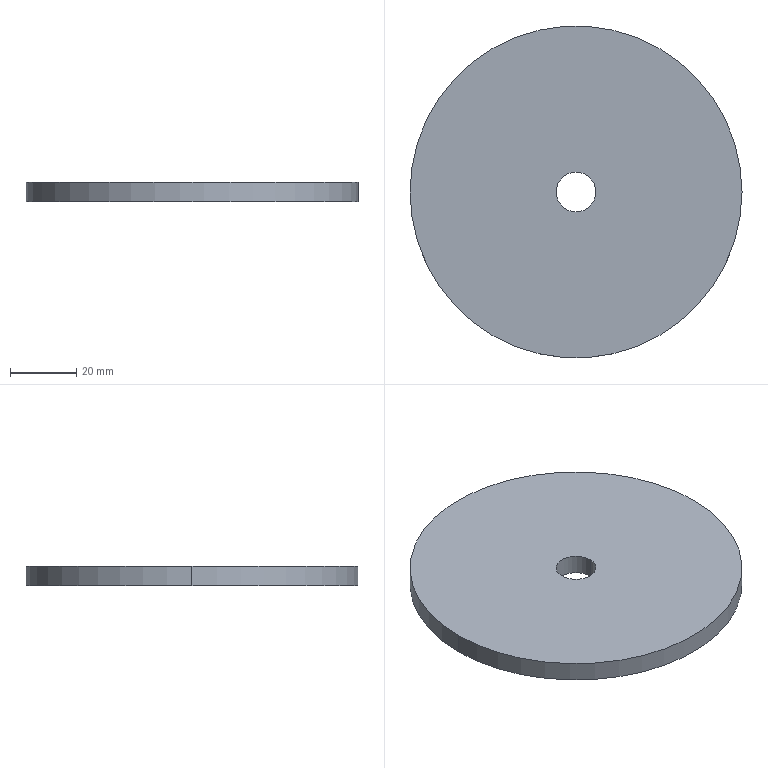Part | SolidWorks | features FlatPattern 1, SMBaseFlange 1, SheetMetal 1 | 1 solid | 6 faces | box 100 x 100 x 6 mm | volume 46445 mm3 | cylinder 4 | plane 2 | commonest cylinder face diameters 12 x2 100 x2
STEP:
#1=CARTESIAN_POINT('',(-1066.,0.,6.));
#2=VERTEX_POINT('',#1);
#3=CARTESIAN_POINT('',(-1054.,0.,6.));
#4=VERTEX_POINT('',#3);
#5=CARTESIAN_POINT('',(-1060.,0.,6.));
#6=DIRECTION('',(0.,0.,1.));
#7=DIRECTION('',(1.,0.,0.));
#8=AXIS2_PLACEMENT_3D('',#5,#6,#7);
#9=CIRCLE('',#8,6.);
#10=EDGE_CURVE('',#2,#4,#9,.T.);
#11=ORIENTED_EDGE('',*,*,#10,.T.);
#12=CARTESIAN_POINT('',(-1054.,0.,0.));
#13=VERTEX_POINT('',#12);
#14=CARTESIAN_POINT('',(-1054.,0.,6.));
#15=DIRECTION('',(0.,0.,-1.));
#16=VECTOR('',#15,1000.);
#17=LINE('',#14,#16);
#18=EDGE_CURVE('',#4,#13,#17,.T.);
#19=ORIENTED_EDGE('',*,*,#18,.T.);
#20=CARTESIAN_POINT('',(-1066.,0.,0.));
#21=VERTEX_POINT('',#20);
#22=CARTESIAN_POINT('',(-1060.,0.,0.));
#23=DIRECTION('',(0.,0.,1.));
#24=DIRECTION('',(1.,0.,0.));
#25=AXIS2_PLACEMENT_3D('',#22,#23,#24);
#26=CIRCLE('',#25,6.);
#27=EDGE_CURVE('',#21,#13,#26,.T.);
#28=ORIENTED_EDGE('',*,*,#27,.F.);
#29=CARTESIAN_POINT('',(-1066.,0.,6.));
#30=DIRECTION('',(0.,0.,-1.));
#31=VECTOR('',#30,1000.);
#32=LINE('',#29,#31);
#33=EDGE_CURVE('',#2,#21,#32,.T.);
#34=ORIENTED_EDGE('',*,*,#33,.F.);
#35=EDGE_LOOP('',(#11,#19,#28,#34));
#36=FACE_OUTER_BOUND('',#35,.T.);
#37=CARTESIAN_POINT('',(-1060.,0.,6.));
#38=DIRECTION('',(0.,0.,-1.));
#39=DIRECTION('',(-1.,0.,0.));
#40=AXIS2_PLACEMENT_3D('',#37,#38,#39);
#41=CYLINDRICAL_SURFACE('',#40,6.);
#42=ADVANCED_FACE('',(#36),#41,.F.);
#43=CARTESIAN_POINT('',(-1010.,0.,6.));
#44=VERTEX_POINT('',#43);
#45=CARTESIAN_POINT('',(-1110.,0.,6.));
#46=VERTEX_POINT('',#45);
#47=CARTESIAN_POINT('',(-1060.,0.,6.));
#48=DIRECTION('',(0.,0.,1.));
#49=DIRECTION('',(1.,0.,0.));
#50=AXIS2_PLACEMENT_3D('',#47,#48,#49);
#51=CIRCLE('',#50,50.);
#52=EDGE_CURVE('',#44,#46,#51,.T.);
#53=ORIENTED_EDGE('',*,*,#52,.F.);
#54=CARTESIAN_POINT('',(-1010.,0.,0.));
#55=VERTEX_POINT('',#54);
#56=CARTESIAN_POINT('',(-1010.,0.,6.));
#57=DIRECTION('',(0.,0.,-1.));
#58=VECTOR('',#57,1000.);
#59=LINE('',#56,#58);
#60=EDGE_CURVE('',#44,#55,#59,.T.);
#61=ORIENTED_EDGE('',*,*,#60,.T.);
#62=CARTESIAN_POINT('',(-1110.,0.,0.));
#63=VERTEX_POINT('',#62);
#64=CARTESIAN_POINT('',(-1060.,0.,0.));
#65=DIRECTION('',(0.,0.,1.));
#66=DIRECTION('',(1.,0.,0.));
#67=AXIS2_PLACEMENT_3D('',#64,#65,#66);
#68=CIRCLE('',#67,50.);
#69=EDGE_CURVE('',#55,#63,#68,.T.);
#70=ORIENTED_EDGE('',*,*,#69,.T.);
#71=CARTESIAN_POINT('',(-1110.,0.,6.));
#72=DIRECTION('',(0.,0.,-1.));
#73=VECTOR('',#72,1000.);
#74=LINE('',#71,#73);
#75=EDGE_CURVE('',#46,#63,#74,.T.);
#76=ORIENTED_EDGE('',*,*,#75,.F.);
#77=EDGE_LOOP('',(#53,#61,#70,#76));
#78=FACE_OUTER_BOUND('',#77,.T.);
#79=CARTESIAN_POINT('',(-1060.,0.,6.));
#80=DIRECTION('',(0.,0.,-1.));
#81=DIRECTION('',(-1.,0.,0.));
#82=AXIS2_PLACEMENT_3D('',#79,#80,#81);
#83=CYLINDRICAL_SURFACE('',#82,50.);
#84=ADVANCED_FACE('',(#78),#83,.T.);
#85=CARTESIAN_POINT('',(-1060.,0.,6.));
#86=DIRECTION('',(0.,0.,1.));
#87=DIRECTION('',(1.,0.,0.));
#88=AXIS2_PLACEMENT_3D('',#85,#86,#87);
#89=CIRCLE('',#88,50.);
#90=EDGE_CURVE('',#46,#44,#89,.T.);
#91=ORIENTED_EDGE('',*,*,#90,.T.);
#92=ORIENTED_EDGE('',*,*,#52,.T.);
#93=EDGE_LOOP('',(#91,#92));
#94=FACE_OUTER_BOUND('',#93,.T.);
#95=ORIENTED_EDGE('',*,*,#10,.F.);
#96=CARTESIAN_POINT('',(-1060.,0.,6.));
#97=DIRECTION('',(0.,0.,1.));
#98=DIRECTION('',(1.,0.,0.));
#99=AXIS2_PLACEMENT_3D('',#96,#97,#98);
#100=CIRCLE('',#99,6.);
#101=EDGE_CURVE('',#4,#2,#100,.T.);
#102=ORIENTED_EDGE('',*,*,#101,.F.);
#103=EDGE_LOOP('',(#95,#102));
#104=FACE_BOUND('',#103,.T.);
#105=CARTESIAN_POINT('',(-1060.,0.,6.));
#106=DIRECTION('',(0.,0.,1.));
#107=DIRECTION('',(1.,0.,0.));
#108=AXIS2_PLACEMENT_3D('',#105,#106,#107);
#109=PLANE('',#108);
#110=ADVANCED_FACE('',(#94,#104),#109,.T.);
#111=CARTESIAN_POINT('',(-1060.,0.,0.));
#112=DIRECTION('',(0.,0.,1.));
#113=DIRECTION('',(1.,0.,0.));
#114=AXIS2_PLACEMENT_3D('',#111,#112,#113);
#115=CIRCLE('',#114,50.);
#116=EDGE_CURVE('',#63,#55,#115,.T.);
#117=ORIENTED_EDGE('',*,*,#116,.F.);
#118=ORIENTED_EDGE('',*,*,#69,.F.);
#119=EDGE_LOOP('',(#117,#118));
#120=FACE_OUTER_BOUND('',#119,.T.);
#121=ORIENTED_EDGE('',*,*,#27,.T.);
#122=CARTESIAN_POINT('',(-1060.,0.,0.));
#123=DIRECTION('',(0.,0.,1.));
#124=DIRECTION('',(1.,0.,0.));
#125=AXIS2_PLACEMENT_3D('',#122,#123,#124);
#126=CIRCLE('',#125,6.);
#127=EDGE_CURVE('',#13,#21,#126,.T.);
#128=ORIENTED_EDGE('',*,*,#127,.T.);
#129=EDGE_LOOP('',(#121,#128));
#130=FACE_BOUND('',#129,.T.);
#131=CARTESIAN_POINT('',(-1060.,0.,0.));
#132=DIRECTION('',(0.,0.,1.));
#133=DIRECTION('',(1.,0.,0.));
#134=AXIS2_PLACEMENT_3D('',#131,#132,#133);
#135=PLANE('',#134);
#136=ADVANCED_FACE('',(#120,#130),#135,.F.);
#137=ORIENTED_EDGE('',*,*,#60,.F.);
#138=ORIENTED_EDGE('',*,*,#90,.F.);
#139=ORIENTED_EDGE('',*,*,#75,.T.);
#140=ORIENTED_EDGE('',*,*,#116,.T.);
#141=EDGE_LOOP('',(#137,#138,#139,#140));
#142=FACE_OUTER_BOUND('',#141,.T.);
#143=CARTESIAN_POINT('',(-1060.,0.,6.));
#144=DIRECTION('',(0.,0.,-1.));
#145=DIRECTION('',(-1.,0.,0.));
#146=AXIS2_PLACEMENT_3D('',#143,#144,#145);
#147=CYLINDRICAL_SURFACE('',#146,50.);
#148=ADVANCED_FACE('',(#142),#147,.T.);
#149=ORIENTED_EDGE('',*,*,#18,.F.);
#150=ORIENTED_EDGE('',*,*,#101,.T.);
#151=ORIENTED_EDGE('',*,*,#33,.T.);
#152=ORIENTED_EDGE('',*,*,#127,.F.);
#153=EDGE_LOOP('',(#149,#150,#151,#152));
#154=FACE_OUTER_BOUND('',#153,.T.);
#155=CARTESIAN_POINT('',(-1060.,0.,6.));
#156=DIRECTION('',(0.,0.,-1.));
#157=DIRECTION('',(-1.,0.,0.));
#158=AXIS2_PLACEMENT_3D('',#155,#156,#157);
#159=CYLINDRICAL_SURFACE('',#158,6.);
#160=ADVANCED_FACE('',(#154),#159,.F.);
#161=CLOSED_SHELL('',(#42,#84,#110,#136,#148,#160));
#162=MANIFOLD_SOLID_BREP('',#161);
#163=CARTESIAN_POINT('',(0.,0.,0.));
#164=DIRECTION('',(0.,0.,1.));
#165=DIRECTION('',(1.,0.,0.));
#166=AXIS2_PLACEMENT_3D('',#163,#164,#165);
#167=(LENGTH_UNIT()NAMED_UNIT(*)SI_UNIT(.MILLI.,.METRE.));
#168=UNCERTAINTY_MEASURE_WITH_UNIT(LENGTH_MEASURE(0.00001),#167,'','');
#169=(NAMED_UNIT(*)PLANE_ANGLE_UNIT()SI_UNIT($,.RADIAN.));
#170=(NAMED_UNIT(*)SI_UNIT($,.STERADIAN.)SOLID_ANGLE_UNIT());
#171=(GEOMETRIC_REPRESENTATION_CONTEXT(3)GLOBAL_UNCERTAINTY_ASSIGNED_CONTEXT((#168))GLOBAL_UNIT_ASSIGNED_CONTEXT((#167,#169,#170))REPRESENTATION_CONTEXT('',''));
#172=ADVANCED_BREP_SHAPE_REPRESENTATION('',(#162,#166),#171);